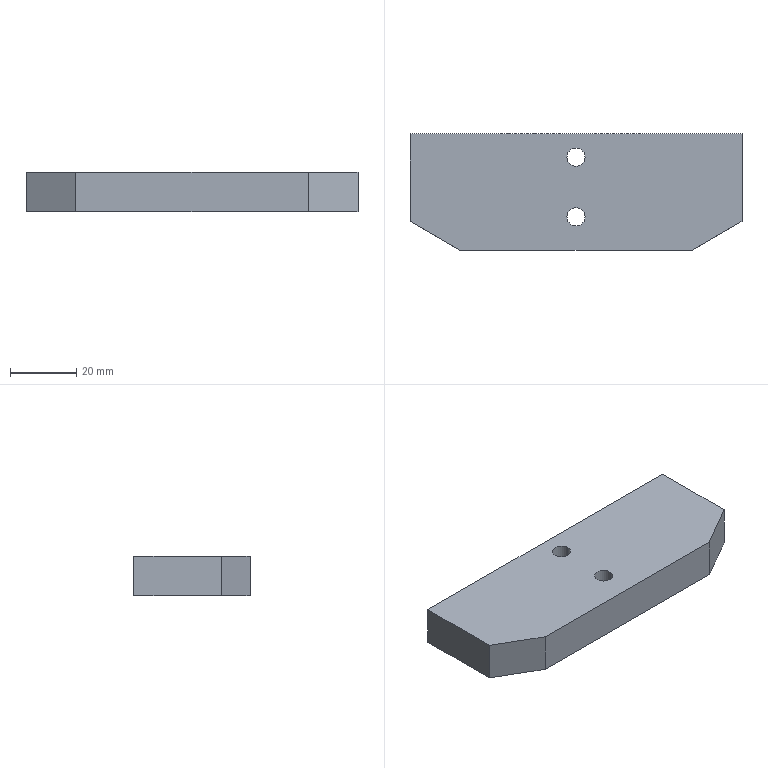Part | SolidWorks | features Chamfer 1, Extrusion 1, HoleWzd 1 | 1 solid | 18 faces | box 100 x 35 x 12 mm | volume 39246 mm3 | plane 10 | cylinder 8 | commonest cylinder face diameters 5.5 x4 10 x4
STEP:
#1=CARTESIAN_POINT('',(5.,10.5,5.7));
#2=VERTEX_POINT('',#1);
#3=CARTESIAN_POINT('',(-5.,10.5,5.7));
#4=VERTEX_POINT('',#3);
#5=CARTESIAN_POINT('',(0.,10.5,5.7));
#6=DIRECTION('',(0.,0.,-1.));
#7=DIRECTION('',(-1.,0.,0.));
#8=AXIS2_PLACEMENT_3D('',#5,#6,#7);
#9=CIRCLE('',#8,5.);
#10=EDGE_CURVE('',#2,#4,#9,.T.);
#11=ORIENTED_EDGE('',*,*,#10,.F.);
#12=CARTESIAN_POINT('',(5.,10.5,0.));
#13=VERTEX_POINT('',#12);
#14=CARTESIAN_POINT('',(5.,10.5,0.));
#15=DIRECTION('',(0.,0.,-1.));
#16=VECTOR('',#15,1000.);
#17=LINE('',#14,#16);
#18=EDGE_CURVE('',#2,#13,#17,.T.);
#19=ORIENTED_EDGE('',*,*,#18,.T.);
#20=CARTESIAN_POINT('',(-5.,10.5,0.));
#21=VERTEX_POINT('',#20);
#22=CARTESIAN_POINT('',(0.,10.5,0.));
#23=DIRECTION('',(0.,0.,-1.));
#24=DIRECTION('',(-1.,0.,0.));
#25=AXIS2_PLACEMENT_3D('',#22,#23,#24);
#26=CIRCLE('',#25,5.);
#27=EDGE_CURVE('',#13,#21,#26,.T.);
#28=ORIENTED_EDGE('',*,*,#27,.T.);
#29=CARTESIAN_POINT('',(-5.,10.5,0.));
#30=DIRECTION('',(0.,0.,-1.));
#31=VECTOR('',#30,1000.);
#32=LINE('',#29,#31);
#33=EDGE_CURVE('',#4,#21,#32,.T.);
#34=ORIENTED_EDGE('',*,*,#33,.F.);
#35=EDGE_LOOP('',(#11,#19,#28,#34));
#36=FACE_OUTER_BOUND('',#35,.T.);
#37=CARTESIAN_POINT('',(0.,10.5,0.));
#38=DIRECTION('',(0.,0.,-1.));
#39=DIRECTION('',(-1.,0.,0.));
#40=AXIS2_PLACEMENT_3D('',#37,#38,#39);
#41=CYLINDRICAL_SURFACE('',#40,5.);
#42=ADVANCED_FACE('',(#36),#41,.F.);
#43=CARTESIAN_POINT('',(-2.75,10.5,12.));
#44=VERTEX_POINT('',#43);
#45=CARTESIAN_POINT('',(2.75,10.5,12.));
#46=VERTEX_POINT('',#45);
#47=CARTESIAN_POINT('',(0.,10.5,12.));
#48=DIRECTION('',(0.,0.,1.));
#49=DIRECTION('',(1.,0.,0.));
#50=AXIS2_PLACEMENT_3D('',#47,#48,#49);
#51=CIRCLE('',#50,2.75);
#52=EDGE_CURVE('',#44,#46,#51,.T.);
#53=ORIENTED_EDGE('',*,*,#52,.T.);
#54=CARTESIAN_POINT('',(2.75,10.5,5.7));
#55=VERTEX_POINT('',#54);
#56=CARTESIAN_POINT('',(2.75,10.5,0.));
#57=DIRECTION('',(0.,0.,-1.));
#58=VECTOR('',#57,1000.);
#59=LINE('',#56,#58);
#60=EDGE_CURVE('',#46,#55,#59,.T.);
#61=ORIENTED_EDGE('',*,*,#60,.T.);
#62=CARTESIAN_POINT('',(-2.75,10.5,5.7));
#63=VERTEX_POINT('',#62);
#64=CARTESIAN_POINT('',(0.,10.5,5.7));
#65=DIRECTION('',(0.,0.,-1.));
#66=DIRECTION('',(-1.,0.,0.));
#67=AXIS2_PLACEMENT_3D('',#64,#65,#66);
#68=CIRCLE('',#67,2.75);
#69=EDGE_CURVE('',#55,#63,#68,.T.);
#70=ORIENTED_EDGE('',*,*,#69,.T.);
#71=CARTESIAN_POINT('',(-2.75,10.5,0.));
#72=DIRECTION('',(0.,0.,-1.));
#73=VECTOR('',#72,1000.);
#74=LINE('',#71,#73);
#75=EDGE_CURVE('',#44,#63,#74,.T.);
#76=ORIENTED_EDGE('',*,*,#75,.F.);
#77=EDGE_LOOP('',(#53,#61,#70,#76));
#78=FACE_OUTER_BOUND('',#77,.T.);
#79=CARTESIAN_POINT('',(0.,10.5,0.));
#80=DIRECTION('',(0.,0.,-1.));
#81=DIRECTION('',(-1.,0.,0.));
#82=AXIS2_PLACEMENT_3D('',#79,#80,#81);
#83=CYLINDRICAL_SURFACE('',#82,2.75);
#84=ADVANCED_FACE('',(#78),#83,.F.);
#85=CARTESIAN_POINT('',(5.,-7.5,5.7));
#86=VERTEX_POINT('',#85);
#87=CARTESIAN_POINT('',(-5.,-7.5,5.7));
#88=VERTEX_POINT('',#87);
#89=CARTESIAN_POINT('',(0.,-7.5,5.7));
#90=DIRECTION('',(0.,0.,-1.));
#91=DIRECTION('',(-1.,0.,0.));
#92=AXIS2_PLACEMENT_3D('',#89,#90,#91);
#93=CIRCLE('',#92,5.);
#94=EDGE_CURVE('',#86,#88,#93,.T.);
#95=ORIENTED_EDGE('',*,*,#94,.F.);
#96=CARTESIAN_POINT('',(5.,-7.5,0.));
#97=VERTEX_POINT('',#96);
#98=CARTESIAN_POINT('',(5.,-7.5,0.));
#99=DIRECTION('',(0.,0.,-1.));
#100=VECTOR('',#99,1000.);
#101=LINE('',#98,#100);
#102=EDGE_CURVE('',#86,#97,#101,.T.);
#103=ORIENTED_EDGE('',*,*,#102,.T.);
#104=CARTESIAN_POINT('',(-5.,-7.5,0.));
#105=VERTEX_POINT('',#104);
#106=CARTESIAN_POINT('',(0.,-7.5,0.));
#107=DIRECTION('',(0.,0.,-1.));
#108=DIRECTION('',(-1.,0.,0.));
#109=AXIS2_PLACEMENT_3D('',#106,#107,#108);
#110=CIRCLE('',#109,5.);
#111=EDGE_CURVE('',#97,#105,#110,.T.);
#112=ORIENTED_EDGE('',*,*,#111,.T.);
#113=CARTESIAN_POINT('',(-5.,-7.5,0.));
#114=DIRECTION('',(0.,0.,-1.));
#115=VECTOR('',#114,1000.);
#116=LINE('',#113,#115);
#117=EDGE_CURVE('',#88,#105,#116,.T.);
#118=ORIENTED_EDGE('',*,*,#117,.F.);
#119=EDGE_LOOP('',(#95,#103,#112,#118));
#120=FACE_OUTER_BOUND('',#119,.T.);
#121=CARTESIAN_POINT('',(0.,-7.5,0.));
#122=DIRECTION('',(0.,0.,-1.));
#123=DIRECTION('',(-1.,0.,0.));
#124=AXIS2_PLACEMENT_3D('',#121,#122,#123);
#125=CYLINDRICAL_SURFACE('',#124,5.);
#126=ADVANCED_FACE('',(#120),#125,.F.);
#127=CARTESIAN_POINT('',(-2.75,-7.5,12.));
#128=VERTEX_POINT('',#127);
#129=CARTESIAN_POINT('',(2.75,-7.5,12.));
#130=VERTEX_POINT('',#129);
#131=CARTESIAN_POINT('',(0.,-7.5,12.));
#132=DIRECTION('',(0.,0.,1.));
#133=DIRECTION('',(1.,0.,0.));
#134=AXIS2_PLACEMENT_3D('',#131,#132,#133);
#135=CIRCLE('',#134,2.75);
#136=EDGE_CURVE('',#128,#130,#135,.T.);
#137=ORIENTED_EDGE('',*,*,#136,.T.);
#138=CARTESIAN_POINT('',(2.75,-7.5,5.7));
#139=VERTEX_POINT('',#138);
#140=CARTESIAN_POINT('',(2.75,-7.5,0.));
#141=DIRECTION('',(0.,0.,-1.));
#142=VECTOR('',#141,1000.);
#143=LINE('',#140,#142);
#144=EDGE_CURVE('',#130,#139,#143,.T.);
#145=ORIENTED_EDGE('',*,*,#144,.T.);
#146=CARTESIAN_POINT('',(-2.75,-7.5,5.7));
#147=VERTEX_POINT('',#146);
#148=CARTESIAN_POINT('',(0.,-7.5,5.7));
#149=DIRECTION('',(0.,0.,-1.));
#150=DIRECTION('',(-1.,0.,0.));
#151=AXIS2_PLACEMENT_3D('',#148,#149,#150);
#152=CIRCLE('',#151,2.75);
#153=EDGE_CURVE('',#139,#147,#152,.T.);
#154=ORIENTED_EDGE('',*,*,#153,.T.);
#155=CARTESIAN_POINT('',(-2.75,-7.5,0.));
#156=DIRECTION('',(0.,0.,-1.));
#157=VECTOR('',#156,1000.);
#158=LINE('',#155,#157);
#159=EDGE_CURVE('',#128,#147,#158,.T.);
#160=ORIENTED_EDGE('',*,*,#159,.F.);
#161=EDGE_LOOP('',(#137,#145,#154,#160));
#162=FACE_OUTER_BOUND('',#161,.T.);
#163=CARTESIAN_POINT('',(0.,-7.5,0.));
#164=DIRECTION('',(0.,0.,-1.));
#165=DIRECTION('',(-1.,0.,0.));
#166=AXIS2_PLACEMENT_3D('',#163,#164,#165);
#167=CYLINDRICAL_SURFACE('',#166,2.75);
#168=ADVANCED_FACE('',(#162),#167,.F.);
#169=CARTESIAN_POINT('',(0.,-7.5,0.));
#170=DIRECTION('',(0.,0.,-1.));
#171=DIRECTION('',(-1.,0.,0.));
#172=AXIS2_PLACEMENT_3D('',#169,#170,#171);
#173=CIRCLE('',#172,5.);
#174=EDGE_CURVE('',#105,#97,#173,.T.);
#175=ORIENTED_EDGE('',*,*,#174,.F.);
#176=ORIENTED_EDGE('',*,*,#111,.F.);
#177=EDGE_LOOP('',(#175,#176));
#178=FACE_BOUND('',#177,.T.);
#179=CARTESIAN_POINT('',(50.,-8.84,0.));
#180=VERTEX_POINT('',#179);
#181=CARTESIAN_POINT('',(50.,17.5,0.));
#182=VERTEX_POINT('',#181);
#183=CARTESIAN_POINT('',(50.,-17.5,0.));
#184=DIRECTION('',(0.,1.,0.));
#185=VECTOR('',#184,1000.);
#186=LINE('',#183,#185);
#187=EDGE_CURVE('',#180,#182,#186,.T.);
#188=ORIENTED_EDGE('',*,*,#187,.F.);
#189=CARTESIAN_POINT('',(35.,-17.5,0.));
#190=VERTEX_POINT('',#189);
#191=CARTESIAN_POINT('',(50.,-8.84,0.));
#192=DIRECTION('',(-0.866,-0.5,0.));
#193=VECTOR('',#192,1000.);
#194=LINE('',#191,#193);
#195=EDGE_CURVE('',#180,#190,#194,.T.);
#196=ORIENTED_EDGE('',*,*,#195,.T.);
#197=CARTESIAN_POINT('',(-35.,-17.5,0.));
#198=VERTEX_POINT('',#197);
#199=CARTESIAN_POINT('',(50.,-17.5,0.));
#200=DIRECTION('',(1.,0.,0.));
#201=VECTOR('',#200,1000.);
#202=LINE('',#199,#201);
#203=EDGE_CURVE('',#198,#190,#202,.T.);
#204=ORIENTED_EDGE('',*,*,#203,.F.);
#205=CARTESIAN_POINT('',(-50.,-8.84,0.));
#206=VERTEX_POINT('',#205);
#207=CARTESIAN_POINT('',(-35.,-17.5,0.));
#208=DIRECTION('',(-0.866,0.5,0.));
#209=VECTOR('',#208,1000.);
#210=LINE('',#207,#209);
#211=EDGE_CURVE('',#198,#206,#210,.T.);
#212=ORIENTED_EDGE('',*,*,#211,.T.);
#213=CARTESIAN_POINT('',(-50.,17.5,0.));
#214=VERTEX_POINT('',#213);
#215=CARTESIAN_POINT('',(-50.,-17.5,0.));
#216=DIRECTION('',(0.,-1.,0.));
#217=VECTOR('',#216,1000.);
#218=LINE('',#215,#217);
#219=EDGE_CURVE('',#214,#206,#218,.T.);
#220=ORIENTED_EDGE('',*,*,#219,.F.);
#221=CARTESIAN_POINT('',(50.,17.5,0.));
#222=DIRECTION('',(-1.,0.,0.));
#223=VECTOR('',#222,1000.);
#224=LINE('',#221,#223);
#225=EDGE_CURVE('',#182,#214,#224,.T.);
#226=ORIENTED_EDGE('',*,*,#225,.F.);
#227=EDGE_LOOP('',(#188,#196,#204,#212,#220,#226));
#228=FACE_OUTER_BOUND('',#227,.T.);
#229=CARTESIAN_POINT('',(0.,10.5,0.));
#230=DIRECTION('',(0.,0.,-1.));
#231=DIRECTION('',(-1.,0.,0.));
#232=AXIS2_PLACEMENT_3D('',#229,#230,#231);
#233=CIRCLE('',#232,5.);
#234=EDGE_CURVE('',#21,#13,#233,.T.);
#235=ORIENTED_EDGE('',*,*,#234,.F.);
#236=ORIENTED_EDGE('',*,*,#27,.F.);
#237=EDGE_LOOP('',(#235,#236));
#238=FACE_BOUND('',#237,.T.);
#239=CARTESIAN_POINT('',(0.,0.,0.));
#240=DIRECTION('',(0.,0.,1.));
#241=DIRECTION('',(1.,0.,0.));
#242=AXIS2_PLACEMENT_3D('',#239,#240,#241);
#243=PLANE('',#242);
#244=ADVANCED_FACE('',(#178,#228,#238),#243,.F.);
#245=ORIENTED_EDGE('',*,*,#219,.T.);
#246=CARTESIAN_POINT('',(-50.,-8.84,12.));
#247=VERTEX_POINT('',#246);
#248=CARTESIAN_POINT('',(-50.,-8.84,12.));
#249=DIRECTION('',(0.,0.,1.));
#250=VECTOR('',#249,1000.);
#251=LINE('',#248,#250);
#252=EDGE_CURVE('',#206,#247,#251,.T.);
#253=ORIENTED_EDGE('',*,*,#252,.T.);
#254=CARTESIAN_POINT('',(-50.,17.5,12.));
#255=VERTEX_POINT('',#254);
#256=CARTESIAN_POINT('',(-50.,-17.5,12.));
#257=DIRECTION('',(0.,-1.,0.));
#258=VECTOR('',#257,1000.);
#259=LINE('',#256,#258);
#260=EDGE_CURVE('',#255,#247,#259,.T.);
#261=ORIENTED_EDGE('',*,*,#260,.F.);
#262=CARTESIAN_POINT('',(-50.,17.5,12.));
#263=DIRECTION('',(0.,0.,-1.));
#264=VECTOR('',#263,1000.);
#265=LINE('',#262,#264);
#266=EDGE_CURVE('',#255,#214,#265,.T.);
#267=ORIENTED_EDGE('',*,*,#266,.T.);
#268=EDGE_LOOP('',(#245,#253,#261,#267));
#269=FACE_OUTER_BOUND('',#268,.T.);
#270=CARTESIAN_POINT('',(-50.,-17.5,12.));
#271=DIRECTION('',(1.,0.,0.));
#272=DIRECTION('',(0.,0.,-1.));
#273=AXIS2_PLACEMENT_3D('',#270,#271,#272);
#274=PLANE('',#273);
#275=ADVANCED_FACE('',(#269),#274,.F.);
#276=ORIENTED_EDGE('',*,*,#203,.T.);
#277=CARTESIAN_POINT('',(35.,-17.5,12.));
#278=VERTEX_POINT('',#277);
#279=CARTESIAN_POINT('',(35.,-17.5,12.));
#280=DIRECTION('',(0.,0.,1.));
#281=VECTOR('',#280,1000.);
#282=LINE('',#279,#281);
#283=EDGE_CURVE('',#190,#278,#282,.T.);
#284=ORIENTED_EDGE('',*,*,#283,.T.);
#285=CARTESIAN_POINT('',(-35.,-17.5,12.));
#286=VERTEX_POINT('',#285);
#287=CARTESIAN_POINT('',(50.,-17.5,12.));
#288=DIRECTION('',(1.,0.,0.));
#289=VECTOR('',#288,1000.);
#290=LINE('',#287,#289);
#291=EDGE_CURVE('',#286,#278,#290,.T.);
#292=ORIENTED_EDGE('',*,*,#291,.F.);
#293=CARTESIAN_POINT('',(-35.,-17.5,12.));
#294=DIRECTION('',(0.,0.,-1.));
#295=VECTOR('',#294,1000.);
#296=LINE('',#293,#295);
#297=EDGE_CURVE('',#286,#198,#296,.T.);
#298=ORIENTED_EDGE('',*,*,#297,.T.);
#299=EDGE_LOOP('',(#276,#284,#292,#298));
#300=FACE_OUTER_BOUND('',#299,.T.);
#301=CARTESIAN_POINT('',(50.,-17.5,12.));
#302=DIRECTION('',(0.,1.,0.));
#303=DIRECTION('',(-1.,0.,0.));
#304=AXIS2_PLACEMENT_3D('',#301,#302,#303);
#305=PLANE('',#304);
#306=ADVANCED_FACE('',(#300),#305,.F.);
#307=CARTESIAN_POINT('',(50.,-8.84,12.));
#308=VERTEX_POINT('',#307);
#309=CARTESIAN_POINT('',(50.,17.5,12.));
#310=VERTEX_POINT('',#309);
#311=CARTESIAN_POINT('',(50.,-17.5,12.));
#312=DIRECTION('',(0.,1.,0.));
#313=VECTOR('',#312,1000.);
#314=LINE('',#311,#313);
#315=EDGE_CURVE('',#308,#310,#314,.T.);
#316=ORIENTED_EDGE('',*,*,#315,.F.);
#317=CARTESIAN_POINT('',(50.,-8.84,12.));
#318=DIRECTION('',(0.,0.,-1.));
#319=VECTOR('',#318,1000.);
#320=LINE('',#317,#319);
#321=EDGE_CURVE('',#308,#180,#320,.T.);
#322=ORIENTED_EDGE('',*,*,#321,.T.);
#323=ORIENTED_EDGE('',*,*,#187,.T.);
#324=CARTESIAN_POINT('',(50.,17.5,12.));
#325=DIRECTION('',(0.,0.,-1.));
#326=VECTOR('',#325,1000.);
#327=LINE('',#324,#326);
#328=EDGE_CURVE('',#310,#182,#327,.T.);
#329=ORIENTED_EDGE('',*,*,#328,.F.);
#330=EDGE_LOOP('',(#316,#322,#323,#329));
#331=FACE_OUTER_BOUND('',#330,.T.);
#332=CARTESIAN_POINT('',(50.,-17.5,12.));
#333=DIRECTION('',(-1.,0.,0.));
#334=DIRECTION('',(0.,0.,1.));
#335=AXIS2_PLACEMENT_3D('',#332,#333,#334);
#336=PLANE('',#335);
#337=ADVANCED_FACE('',(#331),#336,.F.);
#338=ORIENTED_EDGE('',*,*,#225,.T.);
#339=ORIENTED_EDGE('',*,*,#266,.F.);
#340=CARTESIAN_POINT('',(50.,17.5,12.));
#341=DIRECTION('',(-1.,0.,0.));
#342=VECTOR('',#341,1000.);
#343=LINE('',#340,#342);
#344=EDGE_CURVE('',#310,#255,#343,.T.);
#345=ORIENTED_EDGE('',*,*,#344,.F.);
#346=ORIENTED_EDGE('',*,*,#328,.T.);
#347=EDGE_LOOP('',(#338,#339,#345,#346));
#348=FACE_OUTER_BOUND('',#347,.T.);
#349=CARTESIAN_POINT('',(50.,17.5,12.));
#350=DIRECTION('',(0.,-1.,0.));
#351=DIRECTION('',(1.,0.,0.));
#352=AXIS2_PLACEMENT_3D('',#349,#350,#351);
#353=PLANE('',#352);
#354=ADVANCED_FACE('',(#348),#353,.F.);
#355=ORIENTED_EDGE('',*,*,#52,.F.);
#356=CARTESIAN_POINT('',(0.,10.5,12.));
#357=DIRECTION('',(0.,0.,1.));
#358=DIRECTION('',(1.,0.,0.));
#359=AXIS2_PLACEMENT_3D('',#356,#357,#358);
#360=CIRCLE('',#359,2.75);
#361=EDGE_CURVE('',#46,#44,#360,.T.);
#362=ORIENTED_EDGE('',*,*,#361,.F.);
#363=EDGE_LOOP('',(#355,#362));
#364=FACE_BOUND('',#363,.T.);
#365=ORIENTED_EDGE('',*,*,#136,.F.);
#366=CARTESIAN_POINT('',(0.,-7.5,12.));
#367=DIRECTION('',(0.,0.,1.));
#368=DIRECTION('',(1.,0.,0.));
#369=AXIS2_PLACEMENT_3D('',#366,#367,#368);
#370=CIRCLE('',#369,2.75);
#371=EDGE_CURVE('',#130,#128,#370,.T.);
#372=ORIENTED_EDGE('',*,*,#371,.F.);
#373=EDGE_LOOP('',(#365,#372));
#374=FACE_BOUND('',#373,.T.);
#375=ORIENTED_EDGE('',*,*,#291,.T.);
#376=CARTESIAN_POINT('',(16.328,-28.28,12.));
#377=DIRECTION('',(0.866,0.5,0.));
#378=VECTOR('',#377,1000.);
#379=LINE('',#376,#378);
#380=EDGE_CURVE('',#278,#308,#379,.T.);
#381=ORIENTED_EDGE('',*,*,#380,.T.);
#382=ORIENTED_EDGE('',*,*,#315,.T.);
#383=ORIENTED_EDGE('',*,*,#344,.T.);
#384=ORIENTED_EDGE('',*,*,#260,.T.);
#385=CARTESIAN_POINT('',(-16.328,-28.28,12.));
#386=DIRECTION('',(0.866,-0.5,0.));
#387=VECTOR('',#386,1000.);
#388=LINE('',#385,#387);
#389=EDGE_CURVE('',#247,#286,#388,.T.);
#390=ORIENTED_EDGE('',*,*,#389,.T.);
#391=EDGE_LOOP('',(#375,#381,#382,#383,#384,#390));
#392=FACE_OUTER_BOUND('',#391,.T.);
#393=CARTESIAN_POINT('',(0.,0.,12.));
#394=DIRECTION('',(0.,0.,1.));
#395=DIRECTION('',(1.,0.,0.));
#396=AXIS2_PLACEMENT_3D('',#393,#394,#395);
#397=PLANE('',#396);
#398=ADVANCED_FACE('',(#364,#374,#392),#397,.T.);
#399=ORIENTED_EDGE('',*,*,#380,.F.);
#400=ORIENTED_EDGE('',*,*,#283,.F.);
#401=ORIENTED_EDGE('',*,*,#195,.F.);
#402=ORIENTED_EDGE('',*,*,#321,.F.);
#403=EDGE_LOOP('',(#399,#400,#401,#402));
#404=FACE_OUTER_BOUND('',#403,.T.);
#405=CARTESIAN_POINT('',(50.,-8.84,12.));
#406=DIRECTION('',(-0.5,0.866,0.));
#407=DIRECTION('',(0.,0.,-1.));
#408=AXIS2_PLACEMENT_3D('',#405,#406,#407);
#409=PLANE('',#408);
#410=ADVANCED_FACE('',(#404),#409,.F.);
#411=ORIENTED_EDGE('',*,*,#389,.F.);
#412=ORIENTED_EDGE('',*,*,#252,.F.);
#413=ORIENTED_EDGE('',*,*,#211,.F.);
#414=ORIENTED_EDGE('',*,*,#297,.F.);
#415=EDGE_LOOP('',(#411,#412,#413,#414));
#416=FACE_OUTER_BOUND('',#415,.T.);
#417=CARTESIAN_POINT('',(-35.,-17.5,12.));
#418=DIRECTION('',(0.5,0.866,0.));
#419=DIRECTION('',(0.,0.,-1.));
#420=AXIS2_PLACEMENT_3D('',#417,#418,#419);
#421=PLANE('',#420);
#422=ADVANCED_FACE('',(#416),#421,.F.);
#423=ORIENTED_EDGE('',*,*,#144,.F.);
#424=ORIENTED_EDGE('',*,*,#371,.T.);
#425=ORIENTED_EDGE('',*,*,#159,.T.);
#426=CARTESIAN_POINT('',(0.,-7.5,5.7));
#427=DIRECTION('',(0.,0.,-1.));
#428=DIRECTION('',(-1.,0.,0.));
#429=AXIS2_PLACEMENT_3D('',#426,#427,#428);
#430=CIRCLE('',#429,2.75);
#431=EDGE_CURVE('',#147,#139,#430,.T.);
#432=ORIENTED_EDGE('',*,*,#431,.T.);
#433=EDGE_LOOP('',(#423,#424,#425,#432));
#434=FACE_OUTER_BOUND('',#433,.T.);
#435=CARTESIAN_POINT('',(0.,-7.5,0.));
#436=DIRECTION('',(0.,0.,-1.));
#437=DIRECTION('',(-1.,0.,0.));
#438=AXIS2_PLACEMENT_3D('',#435,#436,#437);
#439=CYLINDRICAL_SURFACE('',#438,2.75);
#440=ADVANCED_FACE('',(#434),#439,.F.);
#441=ORIENTED_EDGE('',*,*,#431,.F.);
#442=ORIENTED_EDGE('',*,*,#153,.F.);
#443=EDGE_LOOP('',(#441,#442));
#444=FACE_BOUND('',#443,.T.);
#445=CARTESIAN_POINT('',(0.,-7.5,5.7));
#446=DIRECTION('',(0.,0.,-1.));
#447=DIRECTION('',(-1.,0.,0.));
#448=AXIS2_PLACEMENT_3D('',#445,#446,#447);
#449=CIRCLE('',#448,5.);
#450=EDGE_CURVE('',#88,#86,#449,.T.);
#451=ORIENTED_EDGE('',*,*,#450,.T.);
#452=ORIENTED_EDGE('',*,*,#94,.T.);
#453=EDGE_LOOP('',(#451,#452));
#454=FACE_OUTER_BOUND('',#453,.T.);
#455=CARTESIAN_POINT('',(2.75,-7.5,5.7));
#456=DIRECTION('',(0.,0.,1.));
#457=DIRECTION('',(1.,0.,0.));
#458=AXIS2_PLACEMENT_3D('',#455,#456,#457);
#459=PLANE('',#458);
#460=ADVANCED_FACE('',(#444,#454),#459,.F.);
#461=ORIENTED_EDGE('',*,*,#102,.F.);
#462=ORIENTED_EDGE('',*,*,#450,.F.);
#463=ORIENTED_EDGE('',*,*,#117,.T.);
#464=ORIENTED_EDGE('',*,*,#174,.T.);
#465=EDGE_LOOP('',(#461,#462,#463,#464));
#466=FACE_OUTER_BOUND('',#465,.T.);
#467=CARTESIAN_POINT('',(0.,-7.5,0.));
#468=DIRECTION('',(0.,0.,-1.));
#469=DIRECTION('',(-1.,0.,0.));
#470=AXIS2_PLACEMENT_3D('',#467,#468,#469);
#471=CYLINDRICAL_SURFACE('',#470,5.);
#472=ADVANCED_FACE('',(#466),#471,.F.);
#473=ORIENTED_EDGE('',*,*,#60,.F.);
#474=ORIENTED_EDGE('',*,*,#361,.T.);
#475=ORIENTED_EDGE('',*,*,#75,.T.);
#476=CARTESIAN_POINT('',(0.,10.5,5.7));
#477=DIRECTION('',(0.,0.,-1.));
#478=DIRECTION('',(-1.,0.,0.));
#479=AXIS2_PLACEMENT_3D('',#476,#477,#478);
#480=CIRCLE('',#479,2.75);
#481=EDGE_CURVE('',#63,#55,#480,.T.);
#482=ORIENTED_EDGE('',*,*,#481,.T.);
#483=EDGE_LOOP('',(#473,#474,#475,#482));
#484=FACE_OUTER_BOUND('',#483,.T.);
#485=CARTESIAN_POINT('',(0.,10.5,0.));
#486=DIRECTION('',(0.,0.,-1.));
#487=DIRECTION('',(-1.,0.,0.));
#488=AXIS2_PLACEMENT_3D('',#485,#486,#487);
#489=CYLINDRICAL_SURFACE('',#488,2.75);
#490=ADVANCED_FACE('',(#484),#489,.F.);
#491=ORIENTED_EDGE('',*,*,#481,.F.);
#492=ORIENTED_EDGE('',*,*,#69,.F.);
#493=EDGE_LOOP('',(#491,#492));
#494=FACE_BOUND('',#493,.T.);
#495=CARTESIAN_POINT('',(0.,10.5,5.7));
#496=DIRECTION('',(0.,0.,-1.));
#497=DIRECTION('',(-1.,0.,0.));
#498=AXIS2_PLACEMENT_3D('',#495,#496,#497);
#499=CIRCLE('',#498,5.);
#500=EDGE_CURVE('',#4,#2,#499,.T.);
#501=ORIENTED_EDGE('',*,*,#500,.T.);
#502=ORIENTED_EDGE('',*,*,#10,.T.);
#503=EDGE_LOOP('',(#501,#502));
#504=FACE_OUTER_BOUND('',#503,.T.);
#505=CARTESIAN_POINT('',(2.75,10.5,5.7));
#506=DIRECTION('',(0.,0.,1.));
#507=DIRECTION('',(1.,0.,0.));
#508=AXIS2_PLACEMENT_3D('',#505,#506,#507);
#509=PLANE('',#508);
#510=ADVANCED_FACE('',(#494,#504),#509,.F.);
#511=ORIENTED_EDGE('',*,*,#18,.F.);
#512=ORIENTED_EDGE('',*,*,#500,.F.);
#513=ORIENTED_EDGE('',*,*,#33,.T.);
#514=ORIENTED_EDGE('',*,*,#234,.T.);
#515=EDGE_LOOP('',(#511,#512,#513,#514));
#516=FACE_OUTER_BOUND('',#515,.T.);
#517=CARTESIAN_POINT('',(0.,10.5,0.));
#518=DIRECTION('',(0.,0.,-1.));
#519=DIRECTION('',(-1.,0.,0.));
#520=AXIS2_PLACEMENT_3D('',#517,#518,#519);
#521=CYLINDRICAL_SURFACE('',#520,5.);
#522=ADVANCED_FACE('',(#516),#521,.F.);
#523=CLOSED_SHELL('',(#42,#84,#126,#168,#244,#275,#306,#337,#354,#398,#410,#422,#440,#460,#472,#490,#510,#522));
#524=MANIFOLD_SOLID_BREP('',#523);
#525=CARTESIAN_POINT('',(0.,0.,0.));
#526=DIRECTION('',(0.,0.,1.));
#527=DIRECTION('',(1.,0.,0.));
#528=AXIS2_PLACEMENT_3D('',#525,#526,#527);
#529=(LENGTH_UNIT()NAMED_UNIT(*)SI_UNIT(.MILLI.,.METRE.));
#530=UNCERTAINTY_MEASURE_WITH_UNIT(LENGTH_MEASURE(0.00001),#529,'','');
#531=(NAMED_UNIT(*)PLANE_ANGLE_UNIT()SI_UNIT($,.RADIAN.));
#532=(NAMED_UNIT(*)SI_UNIT($,.STERADIAN.)SOLID_ANGLE_UNIT());
#533=(GEOMETRIC_REPRESENTATION_CONTEXT(3)GLOBAL_UNCERTAINTY_ASSIGNED_CONTEXT((#530))GLOBAL_UNIT_ASSIGNED_CONTEXT((#529,#531,#532))REPRESENTATION_CONTEXT('',''));
#534=ADVANCED_BREP_SHAPE_REPRESENTATION('',(#524,#528),#533);